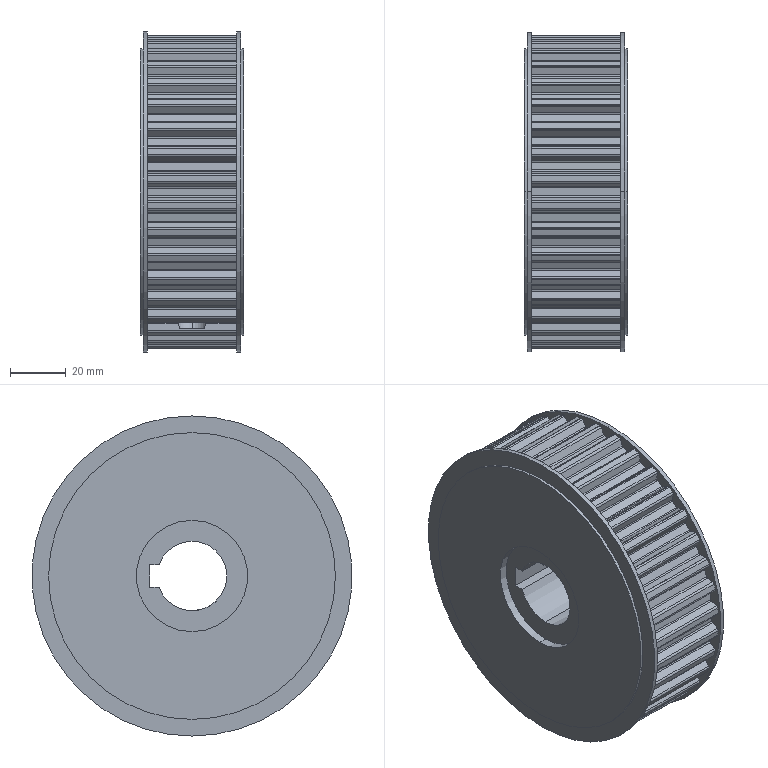Part | SolidWorks | features ICE 8, CirPattern 2, Fillet 2, MirrorPattern 2, Extrusion 1, HoleWzd 1, RevCut 1 | 1 solid | 361 faces | box 37 x 115 x 115 mm | volume 319637 mm3 | cylinder 234 | plane 127 | commonest cylinder face diameters 1.2 x89 1.6 x86 112.74 x36 5 x4 10.5 x4 40 x4